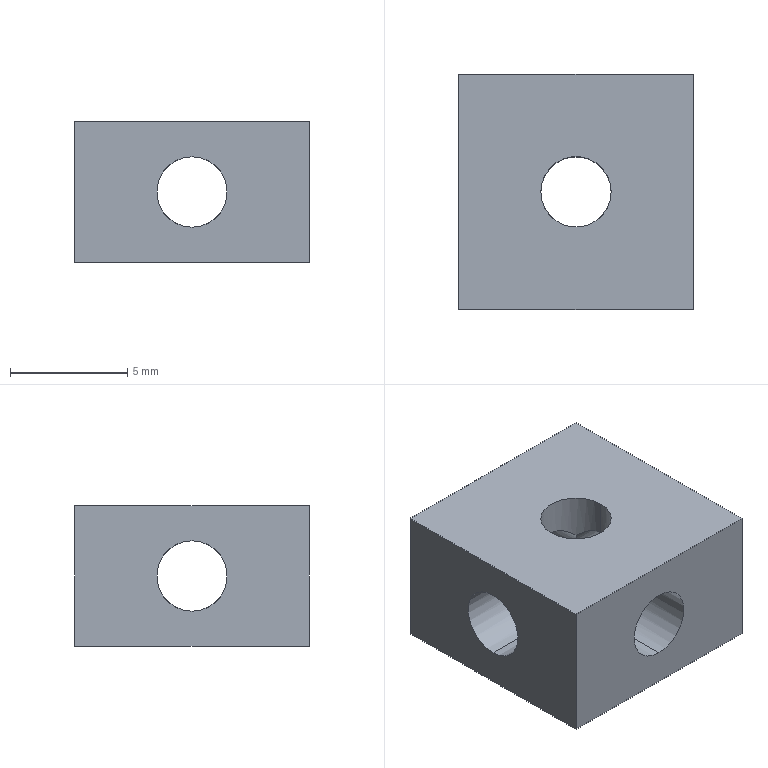Part | SolidWorks | features ICE 3, Extrusion 1 | 1 solid | 18 faces | box 10 x 10 x 6 mm | volume 454.401 mm3 | cylinder 12 | plane 6 | commonest cylinder face diameters 3 x12
STEP:
#1=CARTESIAN_POINT('',(6.5,5.,-1.5));
#2=VERTEX_POINT('',#1);
#3=CARTESIAN_POINT('',(6.061,3.939,-1.939));
#4=VERTEX_POINT('',#3);
#5=CARTESIAN_POINT('',(6.5,5.,-1.5));
#6=CARTESIAN_POINT('',(6.5,4.597,-1.5));
#7=CARTESIAN_POINT('',(6.346,4.224,-1.654));
#8=CARTESIAN_POINT('',(6.061,3.939,-1.939));
#9=(BOUNDED_CURVE()B_SPLINE_CURVE(3,(#5,#6,#7,#8),.UNSPECIFIED.,.F.,.F.)B_SPLINE_CURVE_WITH_KNOTS((4,4),(0.,0.7854),.UNSPECIFIED.)CURVE()GEOMETRIC_REPRESENTATION_ITEM()RATIONAL_B_SPLINE_CURVE((1.,0.9493,0.9493,1.))REPRESENTATION_ITEM(''));
#10=EDGE_CURVE('',#2,#4,#9,.T.);
#11=ORIENTED_EDGE('',*,*,#10,.F.);
#12=CARTESIAN_POINT('',(10.,5.,-1.5));
#13=VERTEX_POINT('',#12);
#14=CARTESIAN_POINT('',(0.,5.,-1.5));
#15=DIRECTION('',(1.,0.,0.));
#16=VECTOR('',#15,1000.);
#17=LINE('',#14,#16);
#18=EDGE_CURVE('',#2,#13,#17,.T.);
#19=ORIENTED_EDGE('',*,*,#18,.T.);
#20=CARTESIAN_POINT('',(10.,5.,-4.5));
#21=VERTEX_POINT('',#20);
#22=CARTESIAN_POINT('',(10.,5.,-3.));
#23=DIRECTION('',(1.,0.,0.));
#24=DIRECTION('',(0.,0.,-1.));
#25=AXIS2_PLACEMENT_3D('',#22,#23,#24);
#26=CIRCLE('',#25,1.5);
#27=EDGE_CURVE('',#13,#21,#26,.T.);
#28=ORIENTED_EDGE('',*,*,#27,.T.);
#29=CARTESIAN_POINT('',(6.5,5.,-4.5));
#30=VERTEX_POINT('',#29);
#31=CARTESIAN_POINT('',(0.,5.,-4.5));
#32=DIRECTION('',(1.,0.,0.));
#33=VECTOR('',#32,1000.);
#34=LINE('',#31,#33);
#35=EDGE_CURVE('',#30,#21,#34,.T.);
#36=ORIENTED_EDGE('',*,*,#35,.F.);
#37=CARTESIAN_POINT('',(6.061,3.939,-4.061));
#38=VERTEX_POINT('',#37);
#39=CARTESIAN_POINT('',(6.061,3.939,-4.061));
#40=CARTESIAN_POINT('',(6.346,4.224,-4.346));
#41=CARTESIAN_POINT('',(6.5,4.597,-4.5));
#42=CARTESIAN_POINT('',(6.5,5.,-4.5));
#43=(BOUNDED_CURVE()B_SPLINE_CURVE(3,(#39,#40,#41,#42),.UNSPECIFIED.,.F.,.F.)B_SPLINE_CURVE_WITH_KNOTS((4,4),(2.356,3.142),.UNSPECIFIED.)CURVE()GEOMETRIC_REPRESENTATION_ITEM()RATIONAL_B_SPLINE_CURVE((1.,0.9493,0.9493,1.))REPRESENTATION_ITEM(''));
#44=EDGE_CURVE('',#38,#30,#43,.T.);
#45=ORIENTED_EDGE('',*,*,#44,.F.);
#46=CARTESIAN_POINT('',(6.061,3.939,-1.939));
#47=CARTESIAN_POINT('',(6.682,3.318,-2.561));
#48=CARTESIAN_POINT('',(6.682,3.318,-3.439));
#49=CARTESIAN_POINT('',(6.061,3.939,-4.061));
#50=(BOUNDED_CURVE()B_SPLINE_CURVE(3,(#46,#47,#48,#49),.UNSPECIFIED.,.F.,.F.)B_SPLINE_CURVE_WITH_KNOTS((4,4),(2.356,3.927),.UNSPECIFIED.)CURVE()GEOMETRIC_REPRESENTATION_ITEM()RATIONAL_B_SPLINE_CURVE((1.,0.8047,0.8047,1.))REPRESENTATION_ITEM(''));
#51=EDGE_CURVE('',#4,#38,#50,.T.);
#52=ORIENTED_EDGE('',*,*,#51,.F.);
#53=EDGE_LOOP('',(#11,#19,#28,#36,#45,#52));
#54=FACE_OUTER_BOUND('',#53,.T.);
#55=CARTESIAN_POINT('',(0.,5.,-3.));
#56=DIRECTION('',(1.,0.,0.));
#57=DIRECTION('',(0.,0.,-1.));
#58=AXIS2_PLACEMENT_3D('',#55,#56,#57);
#59=CYLINDRICAL_SURFACE('',#58,1.5);
#60=ADVANCED_FACE('',(#54),#59,.F.);
#61=CARTESIAN_POINT('',(0.,5.,-1.5));
#62=VERTEX_POINT('',#61);
#63=CARTESIAN_POINT('',(0.,5.,-4.5));
#64=VERTEX_POINT('',#63);
#65=CARTESIAN_POINT('',(0.,5.,-3.));
#66=DIRECTION('',(1.,0.,0.));
#67=DIRECTION('',(0.,0.,-1.));
#68=AXIS2_PLACEMENT_3D('',#65,#66,#67);
#69=CIRCLE('',#68,1.5);
#70=EDGE_CURVE('',#62,#64,#69,.T.);
#71=ORIENTED_EDGE('',*,*,#70,.F.);
#72=CARTESIAN_POINT('',(3.5,5.,-1.5));
#73=VERTEX_POINT('',#72);
#74=CARTESIAN_POINT('',(0.,5.,-1.5));
#75=DIRECTION('',(1.,0.,0.));
#76=VECTOR('',#75,1000.);
#77=LINE('',#74,#76);
#78=EDGE_CURVE('',#62,#73,#77,.T.);
#79=ORIENTED_EDGE('',*,*,#78,.T.);
#80=CARTESIAN_POINT('',(3.939,3.939,-1.939));
#81=VERTEX_POINT('',#80);
#82=CARTESIAN_POINT('',(3.939,3.939,-1.939));
#83=CARTESIAN_POINT('',(3.654,4.224,-1.654));
#84=CARTESIAN_POINT('',(3.5,4.597,-1.5));
#85=CARTESIAN_POINT('',(3.5,5.,-1.5));
#86=(BOUNDED_CURVE()B_SPLINE_CURVE(3,(#82,#83,#84,#85),.UNSPECIFIED.,.F.,.F.)B_SPLINE_CURVE_WITH_KNOTS((4,4),(5.498,6.283),.UNSPECIFIED.)CURVE()GEOMETRIC_REPRESENTATION_ITEM()RATIONAL_B_SPLINE_CURVE((1.,0.9493,0.9493,1.))REPRESENTATION_ITEM(''));
#87=EDGE_CURVE('',#81,#73,#86,.T.);
#88=ORIENTED_EDGE('',*,*,#87,.F.);
#89=CARTESIAN_POINT('',(3.939,3.939,-4.061));
#90=VERTEX_POINT('',#89);
#91=CARTESIAN_POINT('',(3.939,3.939,-4.061));
#92=CARTESIAN_POINT('',(3.318,3.318,-3.439));
#93=CARTESIAN_POINT('',(3.318,3.318,-2.561));
#94=CARTESIAN_POINT('',(3.939,3.939,-1.939));
#95=(BOUNDED_CURVE()B_SPLINE_CURVE(3,(#91,#92,#93,#94),.UNSPECIFIED.,.F.,.F.)B_SPLINE_CURVE_WITH_KNOTS((4,4),(2.356,3.927),.UNSPECIFIED.)CURVE()GEOMETRIC_REPRESENTATION_ITEM()RATIONAL_B_SPLINE_CURVE((1.,0.8047,0.8047,1.))REPRESENTATION_ITEM(''));
#96=EDGE_CURVE('',#90,#81,#95,.T.);
#97=ORIENTED_EDGE('',*,*,#96,.F.);
#98=CARTESIAN_POINT('',(3.5,5.,-4.5));
#99=VERTEX_POINT('',#98);
#100=CARTESIAN_POINT('',(3.5,5.,-4.5));
#101=CARTESIAN_POINT('',(3.5,4.597,-4.5));
#102=CARTESIAN_POINT('',(3.654,4.224,-4.346));
#103=CARTESIAN_POINT('',(3.939,3.939,-4.061));
#104=(BOUNDED_CURVE()B_SPLINE_CURVE(3,(#100,#101,#102,#103),.UNSPECIFIED.,.F.,.T.)B_SPLINE_CURVE_WITH_KNOTS((4,4),(3.142,3.927),.UNSPECIFIED.)CURVE()GEOMETRIC_REPRESENTATION_ITEM()RATIONAL_B_SPLINE_CURVE((1.,0.9493,0.9493,1.))REPRESENTATION_ITEM(''));
#105=EDGE_CURVE('',#99,#90,#104,.T.);
#106=ORIENTED_EDGE('',*,*,#105,.F.);
#107=CARTESIAN_POINT('',(0.,5.,-4.5));
#108=DIRECTION('',(1.,0.,0.));
#109=VECTOR('',#108,1000.);
#110=LINE('',#107,#109);
#111=EDGE_CURVE('',#64,#99,#110,.T.);
#112=ORIENTED_EDGE('',*,*,#111,.F.);
#113=EDGE_LOOP('',(#71,#79,#88,#97,#106,#112));
#114=FACE_OUTER_BOUND('',#113,.T.);
#115=CARTESIAN_POINT('',(0.,5.,-3.));
#116=DIRECTION('',(1.,0.,0.));
#117=DIRECTION('',(0.,0.,-1.));
#118=AXIS2_PLACEMENT_3D('',#115,#116,#117);
#119=CYLINDRICAL_SURFACE('',#118,1.5);
#120=ADVANCED_FACE('',(#114),#119,.F.);
#121=CARTESIAN_POINT('',(5.,0.,-4.5));
#122=VERTEX_POINT('',#121);
#123=CARTESIAN_POINT('',(5.,0.,-1.5));
#124=VERTEX_POINT('',#123);
#125=CARTESIAN_POINT('',(5.,0.,-3.));
#126=DIRECTION('',(0.,1.,0.));
#127=DIRECTION('',(0.,0.,1.));
#128=AXIS2_PLACEMENT_3D('',#125,#126,#127);
#129=CIRCLE('',#128,1.5);
#130=EDGE_CURVE('',#122,#124,#129,.T.);
#131=ORIENTED_EDGE('',*,*,#130,.F.);
#132=CARTESIAN_POINT('',(5.,3.5,-4.5));
#133=VERTEX_POINT('',#132);
#134=CARTESIAN_POINT('',(5.,0.,-4.5));
#135=DIRECTION('',(0.,1.,0.));
#136=VECTOR('',#135,1000.);
#137=LINE('',#134,#136);
#138=EDGE_CURVE('',#122,#133,#137,.T.);
#139=ORIENTED_EDGE('',*,*,#138,.T.);
#140=CARTESIAN_POINT('',(3.939,3.939,-4.061));
#141=CARTESIAN_POINT('',(4.224,3.654,-4.346));
#142=CARTESIAN_POINT('',(4.597,3.5,-4.5));
#143=CARTESIAN_POINT('',(5.,3.5,-4.5));
#144=(BOUNDED_CURVE()B_SPLINE_CURVE(3,(#140,#141,#142,#143),.UNSPECIFIED.,.F.,.F.)B_SPLINE_CURVE_WITH_KNOTS((4,4),(2.356,3.142),.UNSPECIFIED.)CURVE()GEOMETRIC_REPRESENTATION_ITEM()RATIONAL_B_SPLINE_CURVE((1.,0.9493,0.9493,1.))REPRESENTATION_ITEM(''));
#145=EDGE_CURVE('',#90,#133,#144,.T.);
#146=ORIENTED_EDGE('',*,*,#145,.F.);
#147=ORIENTED_EDGE('',*,*,#96,.T.);
#148=CARTESIAN_POINT('',(5.,3.5,-1.5));
#149=VERTEX_POINT('',#148);
#150=CARTESIAN_POINT('',(5.,3.5,-1.5));
#151=CARTESIAN_POINT('',(4.597,3.5,-1.5));
#152=CARTESIAN_POINT('',(4.224,3.654,-1.654));
#153=CARTESIAN_POINT('',(3.939,3.939,-1.939));
#154=(BOUNDED_CURVE()B_SPLINE_CURVE(3,(#150,#151,#152,#153),.UNSPECIFIED.,.F.,.F.)B_SPLINE_CURVE_WITH_KNOTS((4,4),(0.,0.7854),.UNSPECIFIED.)CURVE()GEOMETRIC_REPRESENTATION_ITEM()RATIONAL_B_SPLINE_CURVE((1.,0.9493,0.9493,1.))REPRESENTATION_ITEM(''));
#155=EDGE_CURVE('',#149,#81,#154,.T.);
#156=ORIENTED_EDGE('',*,*,#155,.F.);
#157=CARTESIAN_POINT('',(5.,0.,-1.5));
#158=DIRECTION('',(0.,1.,0.));
#159=VECTOR('',#158,1000.);
#160=LINE('',#157,#159);
#161=EDGE_CURVE('',#124,#149,#160,.T.);
#162=ORIENTED_EDGE('',*,*,#161,.F.);
#163=EDGE_LOOP('',(#131,#139,#146,#147,#156,#162));
#164=FACE_OUTER_BOUND('',#163,.T.);
#165=CARTESIAN_POINT('',(5.,0.,-3.));
#166=DIRECTION('',(0.,1.,0.));
#167=DIRECTION('',(0.,0.,1.));
#168=AXIS2_PLACEMENT_3D('',#165,#166,#167);
#169=CYLINDRICAL_SURFACE('',#168,1.5);
#170=ADVANCED_FACE('',(#164),#169,.F.);
#171=CARTESIAN_POINT('',(5.,6.5,-4.5));
#172=VERTEX_POINT('',#171);
#173=CARTESIAN_POINT('',(3.939,6.061,-4.061));
#174=VERTEX_POINT('',#173);
#175=CARTESIAN_POINT('',(5.,6.5,-4.5));
#176=CARTESIAN_POINT('',(4.597,6.5,-4.5));
#177=CARTESIAN_POINT('',(4.224,6.346,-4.346));
#178=CARTESIAN_POINT('',(3.939,6.061,-4.061));
#179=(BOUNDED_CURVE()B_SPLINE_CURVE(3,(#175,#176,#177,#178),.UNSPECIFIED.,.F.,.F.)B_SPLINE_CURVE_WITH_KNOTS((4,4),(3.142,3.927),.UNSPECIFIED.)CURVE()GEOMETRIC_REPRESENTATION_ITEM()RATIONAL_B_SPLINE_CURVE((1.,0.9493,0.9493,1.))REPRESENTATION_ITEM(''));
#180=EDGE_CURVE('',#172,#174,#179,.T.);
#181=ORIENTED_EDGE('',*,*,#180,.F.);
#182=CARTESIAN_POINT('',(5.,10.,-4.5));
#183=VERTEX_POINT('',#182);
#184=CARTESIAN_POINT('',(5.,0.,-4.5));
#185=DIRECTION('',(0.,1.,0.));
#186=VECTOR('',#185,1000.);
#187=LINE('',#184,#186);
#188=EDGE_CURVE('',#172,#183,#187,.T.);
#189=ORIENTED_EDGE('',*,*,#188,.T.);
#190=CARTESIAN_POINT('',(5.,10.,-1.5));
#191=VERTEX_POINT('',#190);
#192=CARTESIAN_POINT('',(5.,10.,-3.));
#193=DIRECTION('',(0.,1.,0.));
#194=DIRECTION('',(0.,0.,1.));
#195=AXIS2_PLACEMENT_3D('',#192,#193,#194);
#196=CIRCLE('',#195,1.5);
#197=EDGE_CURVE('',#183,#191,#196,.T.);
#198=ORIENTED_EDGE('',*,*,#197,.T.);
#199=CARTESIAN_POINT('',(5.,6.5,-1.5));
#200=VERTEX_POINT('',#199);
#201=CARTESIAN_POINT('',(5.,0.,-1.5));
#202=DIRECTION('',(0.,1.,0.));
#203=VECTOR('',#202,1000.);
#204=LINE('',#201,#203);
#205=EDGE_CURVE('',#200,#191,#204,.T.);
#206=ORIENTED_EDGE('',*,*,#205,.F.);
#207=CARTESIAN_POINT('',(3.939,6.061,-1.939));
#208=VERTEX_POINT('',#207);
#209=CARTESIAN_POINT('',(3.939,6.061,-1.939));
#210=CARTESIAN_POINT('',(4.224,6.346,-1.654));
#211=CARTESIAN_POINT('',(4.597,6.5,-1.5));
#212=CARTESIAN_POINT('',(5.,6.5,-1.5));
#213=(BOUNDED_CURVE()B_SPLINE_CURVE(3,(#209,#210,#211,#212),.UNSPECIFIED.,.F.,.F.)B_SPLINE_CURVE_WITH_KNOTS((4,4),(5.498,6.283),.UNSPECIFIED.)CURVE()GEOMETRIC_REPRESENTATION_ITEM()RATIONAL_B_SPLINE_CURVE((1.,0.9493,0.9493,1.))REPRESENTATION_ITEM(''));
#214=EDGE_CURVE('',#208,#200,#213,.T.);
#215=ORIENTED_EDGE('',*,*,#214,.F.);
#216=CARTESIAN_POINT('',(3.939,6.061,-1.939));
#217=CARTESIAN_POINT('',(3.318,6.682,-2.561));
#218=CARTESIAN_POINT('',(3.318,6.682,-3.439));
#219=CARTESIAN_POINT('',(3.939,6.061,-4.061));
#220=(BOUNDED_CURVE()B_SPLINE_CURVE(3,(#216,#217,#218,#219),.UNSPECIFIED.,.F.,.T.)B_SPLINE_CURVE_WITH_KNOTS((4,4),(5.498,7.069),.UNSPECIFIED.)CURVE()GEOMETRIC_REPRESENTATION_ITEM()RATIONAL_B_SPLINE_CURVE((1.,0.8047,0.8047,1.))REPRESENTATION_ITEM(''));
#221=EDGE_CURVE('',#208,#174,#220,.T.);
#222=ORIENTED_EDGE('',*,*,#221,.T.);
#223=EDGE_LOOP('',(#181,#189,#198,#206,#215,#222));
#224=FACE_OUTER_BOUND('',#223,.T.);
#225=CARTESIAN_POINT('',(5.,0.,-3.));
#226=DIRECTION('',(0.,1.,0.));
#227=DIRECTION('',(0.,0.,1.));
#228=AXIS2_PLACEMENT_3D('',#225,#226,#227);
#229=CYLINDRICAL_SURFACE('',#228,1.5);
#230=ADVANCED_FACE('',(#224),#229,.F.);
#231=CARTESIAN_POINT('',(3.5,5.,-6.));
#232=VERTEX_POINT('',#231);
#233=CARTESIAN_POINT('',(6.5,5.,-6.));
#234=VERTEX_POINT('',#233);
#235=CARTESIAN_POINT('',(5.,5.,-6.));
#236=DIRECTION('',(0.,0.,1.));
#237=DIRECTION('',(1.,0.,0.));
#238=AXIS2_PLACEMENT_3D('',#235,#236,#237);
#239=CIRCLE('',#238,1.5);
#240=EDGE_CURVE('',#232,#234,#239,.T.);
#241=ORIENTED_EDGE('',*,*,#240,.F.);
#242=CARTESIAN_POINT('',(3.5,5.,-6.));
#243=DIRECTION('',(0.,0.,1.));
#244=VECTOR('',#243,1000.);
#245=LINE('',#242,#244);
#246=EDGE_CURVE('',#232,#99,#245,.T.);
#247=ORIENTED_EDGE('',*,*,#246,.T.);
#248=ORIENTED_EDGE('',*,*,#105,.T.);
#249=ORIENTED_EDGE('',*,*,#145,.T.);
#250=CARTESIAN_POINT('',(5.,3.5,-4.5));
#251=CARTESIAN_POINT('',(5.403,3.5,-4.5));
#252=CARTESIAN_POINT('',(5.776,3.654,-4.346));
#253=CARTESIAN_POINT('',(6.061,3.939,-4.061));
#254=(BOUNDED_CURVE()B_SPLINE_CURVE(3,(#250,#251,#252,#253),.UNSPECIFIED.,.F.,.F.)B_SPLINE_CURVE_WITH_KNOTS((4,4),(3.142,3.927),.UNSPECIFIED.)CURVE()GEOMETRIC_REPRESENTATION_ITEM()RATIONAL_B_SPLINE_CURVE((1.,0.9493,0.9493,1.))REPRESENTATION_ITEM(''));
#255=EDGE_CURVE('',#133,#38,#254,.T.);
#256=ORIENTED_EDGE('',*,*,#255,.T.);
#257=ORIENTED_EDGE('',*,*,#44,.T.);
#258=CARTESIAN_POINT('',(6.5,5.,-6.));
#259=DIRECTION('',(0.,0.,1.));
#260=VECTOR('',#259,1000.);
#261=LINE('',#258,#260);
#262=EDGE_CURVE('',#234,#30,#261,.T.);
#263=ORIENTED_EDGE('',*,*,#262,.F.);
#264=EDGE_LOOP('',(#241,#247,#248,#249,#256,#257,#263));
#265=FACE_OUTER_BOUND('',#264,.T.);
#266=CARTESIAN_POINT('',(5.,5.,-6.));
#267=DIRECTION('',(0.,0.,1.));
#268=DIRECTION('',(1.,0.,0.));
#269=AXIS2_PLACEMENT_3D('',#266,#267,#268);
#270=CYLINDRICAL_SURFACE('',#269,1.5);
#271=ADVANCED_FACE('',(#265),#270,.F.);
#272=ORIENTED_EDGE('',*,*,#87,.T.);
#273=CARTESIAN_POINT('',(3.5,5.,0.));
#274=VERTEX_POINT('',#273);
#275=CARTESIAN_POINT('',(3.5,5.,-6.));
#276=DIRECTION('',(0.,0.,1.));
#277=VECTOR('',#276,1000.);
#278=LINE('',#275,#277);
#279=EDGE_CURVE('',#73,#274,#278,.T.);
#280=ORIENTED_EDGE('',*,*,#279,.T.);
#281=CARTESIAN_POINT('',(6.5,5.,0.));
#282=VERTEX_POINT('',#281);
#283=CARTESIAN_POINT('',(5.,5.,0.));
#284=DIRECTION('',(0.,0.,1.));
#285=DIRECTION('',(1.,0.,0.));
#286=AXIS2_PLACEMENT_3D('',#283,#284,#285);
#287=CIRCLE('',#286,1.5);
#288=EDGE_CURVE('',#274,#282,#287,.T.);
#289=ORIENTED_EDGE('',*,*,#288,.T.);
#290=CARTESIAN_POINT('',(6.5,5.,-6.));
#291=DIRECTION('',(0.,0.,1.));
#292=VECTOR('',#291,1000.);
#293=LINE('',#290,#292);
#294=EDGE_CURVE('',#2,#282,#293,.T.);
#295=ORIENTED_EDGE('',*,*,#294,.F.);
#296=ORIENTED_EDGE('',*,*,#10,.T.);
#297=CARTESIAN_POINT('',(6.061,3.939,-1.939));
#298=CARTESIAN_POINT('',(5.776,3.654,-1.654));
#299=CARTESIAN_POINT('',(5.403,3.5,-1.5));
#300=CARTESIAN_POINT('',(5.,3.5,-1.5));
#301=(BOUNDED_CURVE()B_SPLINE_CURVE(3,(#297,#298,#299,#300),.UNSPECIFIED.,.F.,.F.)B_SPLINE_CURVE_WITH_KNOTS((4,4),(5.498,6.283),.UNSPECIFIED.)CURVE()GEOMETRIC_REPRESENTATION_ITEM()RATIONAL_B_SPLINE_CURVE((1.,0.9493,0.9493,1.))REPRESENTATION_ITEM(''));
#302=EDGE_CURVE('',#4,#149,#301,.T.);
#303=ORIENTED_EDGE('',*,*,#302,.T.);
#304=ORIENTED_EDGE('',*,*,#155,.T.);
#305=EDGE_LOOP('',(#272,#280,#289,#295,#296,#303,#304));
#306=FACE_OUTER_BOUND('',#305,.T.);
#307=CARTESIAN_POINT('',(5.,5.,-6.));
#308=DIRECTION('',(0.,0.,1.));
#309=DIRECTION('',(1.,0.,0.));
#310=AXIS2_PLACEMENT_3D('',#307,#308,#309);
#311=CYLINDRICAL_SURFACE('',#310,1.5);
#312=ADVANCED_FACE('',(#306),#311,.F.);
#313=ORIENTED_EDGE('',*,*,#279,.F.);
#314=CARTESIAN_POINT('',(3.5,5.,-1.5));
#315=CARTESIAN_POINT('',(3.5,5.403,-1.5));
#316=CARTESIAN_POINT('',(3.654,5.776,-1.654));
#317=CARTESIAN_POINT('',(3.939,6.061,-1.939));
#318=(BOUNDED_CURVE()B_SPLINE_CURVE(3,(#314,#315,#316,#317),.UNSPECIFIED.,.F.,.T.)B_SPLINE_CURVE_WITH_KNOTS((4,4),(0.,0.7854),.UNSPECIFIED.)CURVE()GEOMETRIC_REPRESENTATION_ITEM()RATIONAL_B_SPLINE_CURVE((1.,0.9493,0.9493,1.))REPRESENTATION_ITEM(''));
#319=EDGE_CURVE('',#73,#208,#318,.T.);
#320=ORIENTED_EDGE('',*,*,#319,.T.);
#321=ORIENTED_EDGE('',*,*,#214,.T.);
#322=CARTESIAN_POINT('',(6.061,6.061,-1.939));
#323=VERTEX_POINT('',#322);
#324=CARTESIAN_POINT('',(5.,6.5,-1.5));
#325=CARTESIAN_POINT('',(5.403,6.5,-1.5));
#326=CARTESIAN_POINT('',(5.776,6.346,-1.654));
#327=CARTESIAN_POINT('',(6.061,6.061,-1.939));
#328=(BOUNDED_CURVE()B_SPLINE_CURVE(3,(#324,#325,#326,#327),.UNSPECIFIED.,.F.,.F.)B_SPLINE_CURVE_WITH_KNOTS((4,4),(0.,0.7854),.UNSPECIFIED.)CURVE()GEOMETRIC_REPRESENTATION_ITEM()RATIONAL_B_SPLINE_CURVE((1.,0.9493,0.9493,1.))REPRESENTATION_ITEM(''));
#329=EDGE_CURVE('',#200,#323,#328,.T.);
#330=ORIENTED_EDGE('',*,*,#329,.T.);
#331=CARTESIAN_POINT('',(6.061,6.061,-1.939));
#332=CARTESIAN_POINT('',(6.346,5.776,-1.654));
#333=CARTESIAN_POINT('',(6.5,5.403,-1.5));
#334=CARTESIAN_POINT('',(6.5,5.,-1.5));
#335=(BOUNDED_CURVE()B_SPLINE_CURVE(3,(#331,#332,#333,#334),.UNSPECIFIED.,.F.,.F.)B_SPLINE_CURVE_WITH_KNOTS((4,4),(5.498,6.283),.UNSPECIFIED.)CURVE()GEOMETRIC_REPRESENTATION_ITEM()RATIONAL_B_SPLINE_CURVE((1.,0.9493,0.9493,1.))REPRESENTATION_ITEM(''));
#336=EDGE_CURVE('',#323,#2,#335,.T.);
#337=ORIENTED_EDGE('',*,*,#336,.T.);
#338=ORIENTED_EDGE('',*,*,#294,.T.);
#339=CARTESIAN_POINT('',(5.,5.,0.));
#340=DIRECTION('',(0.,0.,1.));
#341=DIRECTION('',(1.,0.,0.));
#342=AXIS2_PLACEMENT_3D('',#339,#340,#341);
#343=CIRCLE('',#342,1.5);
#344=EDGE_CURVE('',#282,#274,#343,.T.);
#345=ORIENTED_EDGE('',*,*,#344,.T.);
#346=EDGE_LOOP('',(#313,#320,#321,#330,#337,#338,#345));
#347=FACE_OUTER_BOUND('',#346,.T.);
#348=CARTESIAN_POINT('',(5.,5.,-6.));
#349=DIRECTION('',(0.,0.,1.));
#350=DIRECTION('',(1.,0.,0.));
#351=AXIS2_PLACEMENT_3D('',#348,#349,#350);
#352=CYLINDRICAL_SURFACE('',#351,1.5);
#353=ADVANCED_FACE('',(#347),#352,.F.);
#354=CARTESIAN_POINT('',(0.,5.,-3.));
#355=DIRECTION('',(1.,0.,0.));
#356=DIRECTION('',(0.,0.,-1.));
#357=AXIS2_PLACEMENT_3D('',#354,#355,#356);
#358=CIRCLE('',#357,1.5);
#359=EDGE_CURVE('',#64,#62,#358,.T.);
#360=ORIENTED_EDGE('',*,*,#359,.T.);
#361=ORIENTED_EDGE('',*,*,#70,.T.);
#362=EDGE_LOOP('',(#360,#361));
#363=FACE_BOUND('',#362,.T.);
#364=CARTESIAN_POINT('',(0.,0.,-6.));
#365=VERTEX_POINT('',#364);
#366=CARTESIAN_POINT('',(0.,0.,0.));
#367=VERTEX_POINT('',#366);
#368=CARTESIAN_POINT('',(0.,0.,0.));
#369=DIRECTION('',(0.,0.,1.));
#370=VECTOR('',#369,1000.);
#371=LINE('',#368,#370);
#372=EDGE_CURVE('',#365,#367,#371,.T.);
#373=ORIENTED_EDGE('',*,*,#372,.T.);
#374=CARTESIAN_POINT('',(0.,10.,0.));
#375=VERTEX_POINT('',#374);
#376=CARTESIAN_POINT('',(0.,10.,0.));
#377=DIRECTION('',(0.,-1.,0.));
#378=VECTOR('',#377,1000.);
#379=LINE('',#376,#378);
#380=EDGE_CURVE('',#375,#367,#379,.T.);
#381=ORIENTED_EDGE('',*,*,#380,.F.);
#382=CARTESIAN_POINT('',(0.,10.,-6.));
#383=VERTEX_POINT('',#382);
#384=CARTESIAN_POINT('',(0.,10.,0.));
#385=DIRECTION('',(0.,0.,1.));
#386=VECTOR('',#385,1000.);
#387=LINE('',#384,#386);
#388=EDGE_CURVE('',#383,#375,#387,.T.);
#389=ORIENTED_EDGE('',*,*,#388,.F.);
#390=CARTESIAN_POINT('',(0.,10.,-6.));
#391=DIRECTION('',(0.,-1.,0.));
#392=VECTOR('',#391,1000.);
#393=LINE('',#390,#392);
#394=EDGE_CURVE('',#383,#365,#393,.T.);
#395=ORIENTED_EDGE('',*,*,#394,.T.);
#396=EDGE_LOOP('',(#373,#381,#389,#395));
#397=FACE_OUTER_BOUND('',#396,.T.);
#398=CARTESIAN_POINT('',(0.,10.,0.));
#399=DIRECTION('',(1.,0.,0.));
#400=DIRECTION('',(0.,0.,-1.));
#401=AXIS2_PLACEMENT_3D('',#398,#399,#400);
#402=PLANE('',#401);
#403=ADVANCED_FACE('',(#363,#397),#402,.F.);
#404=ORIENTED_EDGE('',*,*,#344,.F.);
#405=ORIENTED_EDGE('',*,*,#288,.F.);
#406=EDGE_LOOP('',(#404,#405));
#407=FACE_BOUND('',#406,.T.);
#408=CARTESIAN_POINT('',(10.,0.,0.));
#409=VERTEX_POINT('',#408);
#410=CARTESIAN_POINT('',(0.,0.,0.));
#411=DIRECTION('',(1.,0.,0.));
#412=VECTOR('',#411,1000.);
#413=LINE('',#410,#412);
#414=EDGE_CURVE('',#367,#409,#413,.T.);
#415=ORIENTED_EDGE('',*,*,#414,.T.);
#416=CARTESIAN_POINT('',(10.,10.,0.));
#417=VERTEX_POINT('',#416);
#418=CARTESIAN_POINT('',(10.,10.,0.));
#419=DIRECTION('',(0.,-1.,0.));
#420=VECTOR('',#419,1000.);
#421=LINE('',#418,#420);
#422=EDGE_CURVE('',#417,#409,#421,.T.);
#423=ORIENTED_EDGE('',*,*,#422,.F.);
#424=CARTESIAN_POINT('',(0.,10.,0.));
#425=DIRECTION('',(1.,0.,0.));
#426=VECTOR('',#425,1000.);
#427=LINE('',#424,#426);
#428=EDGE_CURVE('',#375,#417,#427,.T.);
#429=ORIENTED_EDGE('',*,*,#428,.F.);
#430=ORIENTED_EDGE('',*,*,#380,.T.);
#431=EDGE_LOOP('',(#415,#423,#429,#430));
#432=FACE_OUTER_BOUND('',#431,.T.);
#433=CARTESIAN_POINT('',(0.,10.,0.));
#434=DIRECTION('',(0.,0.,-1.));
#435=DIRECTION('',(-1.,0.,0.));
#436=AXIS2_PLACEMENT_3D('',#433,#434,#435);
#437=PLANE('',#436);
#438=ADVANCED_FACE('',(#407,#432),#437,.F.);
#439=CARTESIAN_POINT('',(10.,5.,-3.));
#440=DIRECTION('',(1.,0.,0.));
#441=DIRECTION('',(0.,0.,-1.));
#442=AXIS2_PLACEMENT_3D('',#439,#440,#441);
#443=CIRCLE('',#442,1.5);
#444=EDGE_CURVE('',#21,#13,#443,.T.);
#445=ORIENTED_EDGE('',*,*,#444,.F.);
#446=ORIENTED_EDGE('',*,*,#27,.F.);
#447=EDGE_LOOP('',(#445,#446));
#448=FACE_BOUND('',#447,.T.);
#449=CARTESIAN_POINT('',(10.,0.,-6.));
#450=VERTEX_POINT('',#449);
#451=CARTESIAN_POINT('',(10.,0.,0.));
#452=DIRECTION('',(0.,0.,-1.));
#453=VECTOR('',#452,1000.);
#454=LINE('',#451,#453);
#455=EDGE_CURVE('',#409,#450,#454,.T.);
#456=ORIENTED_EDGE('',*,*,#455,.T.);
#457=CARTESIAN_POINT('',(10.,10.,-6.));
#458=VERTEX_POINT('',#457);
#459=CARTESIAN_POINT('',(10.,10.,-6.));
#460=DIRECTION('',(0.,-1.,0.));
#461=VECTOR('',#460,1000.);
#462=LINE('',#459,#461);
#463=EDGE_CURVE('',#458,#450,#462,.T.);
#464=ORIENTED_EDGE('',*,*,#463,.F.);
#465=CARTESIAN_POINT('',(10.,10.,0.));
#466=DIRECTION('',(0.,0.,-1.));
#467=VECTOR('',#466,1000.);
#468=LINE('',#465,#467);
#469=EDGE_CURVE('',#417,#458,#468,.T.);
#470=ORIENTED_EDGE('',*,*,#469,.F.);
#471=ORIENTED_EDGE('',*,*,#422,.T.);
#472=EDGE_LOOP('',(#456,#464,#470,#471));
#473=FACE_OUTER_BOUND('',#472,.T.);
#474=CARTESIAN_POINT('',(10.,10.,0.));
#475=DIRECTION('',(-1.,0.,0.));
#476=DIRECTION('',(0.,0.,1.));
#477=AXIS2_PLACEMENT_3D('',#474,#475,#476);
#478=PLANE('',#477);
#479=ADVANCED_FACE('',(#448,#473),#478,.F.);
#480=CARTESIAN_POINT('',(5.,5.,-6.));
#481=DIRECTION('',(0.,0.,1.));
#482=DIRECTION('',(1.,0.,0.));
#483=AXIS2_PLACEMENT_3D('',#480,#481,#482);
#484=CIRCLE('',#483,1.5);
#485=EDGE_CURVE('',#234,#232,#484,.T.);
#486=ORIENTED_EDGE('',*,*,#485,.T.);
#487=ORIENTED_EDGE('',*,*,#240,.T.);
#488=EDGE_LOOP('',(#486,#487));
#489=FACE_BOUND('',#488,.T.);
#490=CARTESIAN_POINT('',(0.,0.,-6.));
#491=DIRECTION('',(-1.,0.,0.));
#492=VECTOR('',#491,1000.);
#493=LINE('',#490,#492);
#494=EDGE_CURVE('',#450,#365,#493,.T.);
#495=ORIENTED_EDGE('',*,*,#494,.T.);
#496=ORIENTED_EDGE('',*,*,#394,.F.);
#497=CARTESIAN_POINT('',(0.,10.,-6.));
#498=DIRECTION('',(-1.,0.,0.));
#499=VECTOR('',#498,1000.);
#500=LINE('',#497,#499);
#501=EDGE_CURVE('',#458,#383,#500,.T.);
#502=ORIENTED_EDGE('',*,*,#501,.F.);
#503=ORIENTED_EDGE('',*,*,#463,.T.);
#504=EDGE_LOOP('',(#495,#496,#502,#503));
#505=FACE_OUTER_BOUND('',#504,.T.);
#506=CARTESIAN_POINT('',(0.,10.,-6.));
#507=DIRECTION('',(0.,0.,1.));
#508=DIRECTION('',(1.,0.,0.));
#509=AXIS2_PLACEMENT_3D('',#506,#507,#508);
#510=PLANE('',#509);
#511=ADVANCED_FACE('',(#489,#505),#510,.F.);
#512=CARTESIAN_POINT('',(5.,10.,-3.));
#513=DIRECTION('',(0.,1.,0.));
#514=DIRECTION('',(0.,0.,1.));
#515=AXIS2_PLACEMENT_3D('',#512,#513,#514);
#516=CIRCLE('',#515,1.5);
#517=EDGE_CURVE('',#191,#183,#516,.T.);
#518=ORIENTED_EDGE('',*,*,#517,.F.);
#519=ORIENTED_EDGE('',*,*,#197,.F.);
#520=EDGE_LOOP('',(#518,#519));
#521=FACE_BOUND('',#520,.T.);
#522=ORIENTED_EDGE('',*,*,#388,.T.);
#523=ORIENTED_EDGE('',*,*,#428,.T.);
#524=ORIENTED_EDGE('',*,*,#469,.T.);
#525=ORIENTED_EDGE('',*,*,#501,.T.);
#526=EDGE_LOOP('',(#522,#523,#524,#525));
#527=FACE_OUTER_BOUND('',#526,.T.);
#528=CARTESIAN_POINT('',(0.,10.,0.));
#529=DIRECTION('',(0.,-1.,0.));
#530=DIRECTION('',(0.,0.,-1.));
#531=AXIS2_PLACEMENT_3D('',#528,#529,#530);
#532=PLANE('',#531);
#533=ADVANCED_FACE('',(#521,#527),#532,.F.);
#534=CARTESIAN_POINT('',(5.,0.,-3.));
#535=DIRECTION('',(0.,1.,0.));
#536=DIRECTION('',(0.,0.,1.));
#537=AXIS2_PLACEMENT_3D('',#534,#535,#536);
#538=CIRCLE('',#537,1.5);
#539=EDGE_CURVE('',#124,#122,#538,.T.);
#540=ORIENTED_EDGE('',*,*,#539,.T.);
#541=ORIENTED_EDGE('',*,*,#130,.T.);
#542=EDGE_LOOP('',(#540,#541));
#543=FACE_BOUND('',#542,.T.);
#544=ORIENTED_EDGE('',*,*,#372,.F.);
#545=ORIENTED_EDGE('',*,*,#494,.F.);
#546=ORIENTED_EDGE('',*,*,#455,.F.);
#547=ORIENTED_EDGE('',*,*,#414,.F.);
#548=EDGE_LOOP('',(#544,#545,#546,#547));
#549=FACE_OUTER_BOUND('',#548,.T.);
#550=CARTESIAN_POINT('',(0.,0.,0.));
#551=DIRECTION('',(0.,-1.,0.));
#552=DIRECTION('',(0.,0.,-1.));
#553=AXIS2_PLACEMENT_3D('',#550,#551,#552);
#554=PLANE('',#553);
#555=ADVANCED_FACE('',(#543,#549),#554,.T.);
#556=ORIENTED_EDGE('',*,*,#246,.F.);
#557=ORIENTED_EDGE('',*,*,#485,.F.);
#558=ORIENTED_EDGE('',*,*,#262,.T.);
#559=CARTESIAN_POINT('',(6.061,6.061,-4.061));
#560=VERTEX_POINT('',#559);
#561=CARTESIAN_POINT('',(6.5,5.,-4.5));
#562=CARTESIAN_POINT('',(6.5,5.403,-4.5));
#563=CARTESIAN_POINT('',(6.346,5.776,-4.346));
#564=CARTESIAN_POINT('',(6.061,6.061,-4.061));
#565=(BOUNDED_CURVE()B_SPLINE_CURVE(3,(#561,#562,#563,#564),.UNSPECIFIED.,.F.,.F.)B_SPLINE_CURVE_WITH_KNOTS((4,4),(3.142,3.927),.UNSPECIFIED.)CURVE()GEOMETRIC_REPRESENTATION_ITEM()RATIONAL_B_SPLINE_CURVE((1.,0.9493,0.9493,1.))REPRESENTATION_ITEM(''));
#566=EDGE_CURVE('',#30,#560,#565,.T.);
#567=ORIENTED_EDGE('',*,*,#566,.T.);
#568=CARTESIAN_POINT('',(6.061,6.061,-4.061));
#569=CARTESIAN_POINT('',(5.776,6.346,-4.346));
#570=CARTESIAN_POINT('',(5.403,6.5,-4.5));
#571=CARTESIAN_POINT('',(5.,6.5,-4.5));
#572=(BOUNDED_CURVE()B_SPLINE_CURVE(3,(#568,#569,#570,#571),.UNSPECIFIED.,.F.,.F.)B_SPLINE_CURVE_WITH_KNOTS((4,4),(2.356,3.142),.UNSPECIFIED.)CURVE()GEOMETRIC_REPRESENTATION_ITEM()RATIONAL_B_SPLINE_CURVE((1.,0.9493,0.9493,1.))REPRESENTATION_ITEM(''));
#573=EDGE_CURVE('',#560,#172,#572,.T.);
#574=ORIENTED_EDGE('',*,*,#573,.T.);
#575=ORIENTED_EDGE('',*,*,#180,.T.);
#576=CARTESIAN_POINT('',(3.939,6.061,-4.061));
#577=CARTESIAN_POINT('',(3.654,5.776,-4.346));
#578=CARTESIAN_POINT('',(3.5,5.403,-4.5));
#579=CARTESIAN_POINT('',(3.5,5.,-4.5));
#580=(BOUNDED_CURVE()B_SPLINE_CURVE(3,(#576,#577,#578,#579),.UNSPECIFIED.,.F.,.F.)B_SPLINE_CURVE_WITH_KNOTS((4,4),(2.356,3.142),.UNSPECIFIED.)CURVE()GEOMETRIC_REPRESENTATION_ITEM()RATIONAL_B_SPLINE_CURVE((1.,0.9493,0.9493,1.))REPRESENTATION_ITEM(''));
#581=EDGE_CURVE('',#174,#99,#580,.T.);
#582=ORIENTED_EDGE('',*,*,#581,.T.);
#583=EDGE_LOOP('',(#556,#557,#558,#567,#574,#575,#582));
#584=FACE_OUTER_BOUND('',#583,.T.);
#585=CARTESIAN_POINT('',(5.,5.,-6.));
#586=DIRECTION('',(0.,0.,1.));
#587=DIRECTION('',(1.,0.,0.));
#588=AXIS2_PLACEMENT_3D('',#585,#586,#587);
#589=CYLINDRICAL_SURFACE('',#588,1.5);
#590=ADVANCED_FACE('',(#584),#589,.F.);
#591=ORIENTED_EDGE('',*,*,#188,.F.);
#592=ORIENTED_EDGE('',*,*,#573,.F.);
#593=CARTESIAN_POINT('',(6.061,6.061,-4.061));
#594=CARTESIAN_POINT('',(6.682,6.682,-3.439));
#595=CARTESIAN_POINT('',(6.682,6.682,-2.561));
#596=CARTESIAN_POINT('',(6.061,6.061,-1.939));
#597=(BOUNDED_CURVE()B_SPLINE_CURVE(3,(#593,#594,#595,#596),.UNSPECIFIED.,.F.,.F.)B_SPLINE_CURVE_WITH_KNOTS((4,4),(5.498,7.069),.UNSPECIFIED.)CURVE()GEOMETRIC_REPRESENTATION_ITEM()RATIONAL_B_SPLINE_CURVE((1.,0.8047,0.8047,1.))REPRESENTATION_ITEM(''));
#598=EDGE_CURVE('',#560,#323,#597,.T.);
#599=ORIENTED_EDGE('',*,*,#598,.T.);
#600=ORIENTED_EDGE('',*,*,#329,.F.);
#601=ORIENTED_EDGE('',*,*,#205,.T.);
#602=ORIENTED_EDGE('',*,*,#517,.T.);
#603=EDGE_LOOP('',(#591,#592,#599,#600,#601,#602));
#604=FACE_OUTER_BOUND('',#603,.T.);
#605=CARTESIAN_POINT('',(5.,0.,-3.));
#606=DIRECTION('',(0.,1.,0.));
#607=DIRECTION('',(0.,0.,1.));
#608=AXIS2_PLACEMENT_3D('',#605,#606,#607);
#609=CYLINDRICAL_SURFACE('',#608,1.5);
#610=ADVANCED_FACE('',(#604),#609,.F.);
#611=ORIENTED_EDGE('',*,*,#138,.F.);
#612=ORIENTED_EDGE('',*,*,#539,.F.);
#613=ORIENTED_EDGE('',*,*,#161,.T.);
#614=ORIENTED_EDGE('',*,*,#302,.F.);
#615=ORIENTED_EDGE('',*,*,#51,.T.);
#616=ORIENTED_EDGE('',*,*,#255,.F.);
#617=EDGE_LOOP('',(#611,#612,#613,#614,#615,#616));
#618=FACE_OUTER_BOUND('',#617,.T.);
#619=CARTESIAN_POINT('',(5.,0.,-3.));
#620=DIRECTION('',(0.,1.,0.));
#621=DIRECTION('',(0.,0.,1.));
#622=AXIS2_PLACEMENT_3D('',#619,#620,#621);
#623=CYLINDRICAL_SURFACE('',#622,1.5);
#624=ADVANCED_FACE('',(#618),#623,.F.);
#625=ORIENTED_EDGE('',*,*,#78,.F.);
#626=ORIENTED_EDGE('',*,*,#359,.F.);
#627=ORIENTED_EDGE('',*,*,#111,.T.);
#628=ORIENTED_EDGE('',*,*,#581,.F.);
#629=ORIENTED_EDGE('',*,*,#221,.F.);
#630=ORIENTED_EDGE('',*,*,#319,.F.);
#631=EDGE_LOOP('',(#625,#626,#627,#628,#629,#630));
#632=FACE_OUTER_BOUND('',#631,.T.);
#633=CARTESIAN_POINT('',(0.,5.,-3.));
#634=DIRECTION('',(1.,0.,0.));
#635=DIRECTION('',(0.,0.,-1.));
#636=AXIS2_PLACEMENT_3D('',#633,#634,#635);
#637=CYLINDRICAL_SURFACE('',#636,1.5);
#638=ADVANCED_FACE('',(#632),#637,.F.);
#639=ORIENTED_EDGE('',*,*,#18,.F.);
#640=ORIENTED_EDGE('',*,*,#336,.F.);
#641=ORIENTED_EDGE('',*,*,#598,.F.);
#642=ORIENTED_EDGE('',*,*,#566,.F.);
#643=ORIENTED_EDGE('',*,*,#35,.T.);
#644=ORIENTED_EDGE('',*,*,#444,.T.);
#645=EDGE_LOOP('',(#639,#640,#641,#642,#643,#644));
#646=FACE_OUTER_BOUND('',#645,.T.);
#647=CARTESIAN_POINT('',(0.,5.,-3.));
#648=DIRECTION('',(1.,0.,0.));
#649=DIRECTION('',(0.,0.,-1.));
#650=AXIS2_PLACEMENT_3D('',#647,#648,#649);
#651=CYLINDRICAL_SURFACE('',#650,1.5);
#652=ADVANCED_FACE('',(#646),#651,.F.);
#653=CLOSED_SHELL('',(#60,#120,#170,#230,#271,#312,#353,#403,#438,#479,#511,#533,#555,#590,#610,#624,#638,#652));
#654=MANIFOLD_SOLID_BREP('',#653);
#655=CARTESIAN_POINT('',(0.,0.,0.));
#656=DIRECTION('',(0.,0.,1.));
#657=DIRECTION('',(1.,0.,0.));
#658=AXIS2_PLACEMENT_3D('',#655,#656,#657);
#659=(LENGTH_UNIT()NAMED_UNIT(*)SI_UNIT(.MILLI.,.METRE.));
#660=UNCERTAINTY_MEASURE_WITH_UNIT(LENGTH_MEASURE(0.00001),#659,'','');
#661=(NAMED_UNIT(*)PLANE_ANGLE_UNIT()SI_UNIT($,.RADIAN.));
#662=(NAMED_UNIT(*)SI_UNIT($,.STERADIAN.)SOLID_ANGLE_UNIT());
#663=(GEOMETRIC_REPRESENTATION_CONTEXT(3)GLOBAL_UNCERTAINTY_ASSIGNED_CONTEXT((#660))GLOBAL_UNIT_ASSIGNED_CONTEXT((#659,#661,#662))REPRESENTATION_CONTEXT('',''));
#664=ADVANCED_BREP_SHAPE_REPRESENTATION('',(#654,#658),#663);